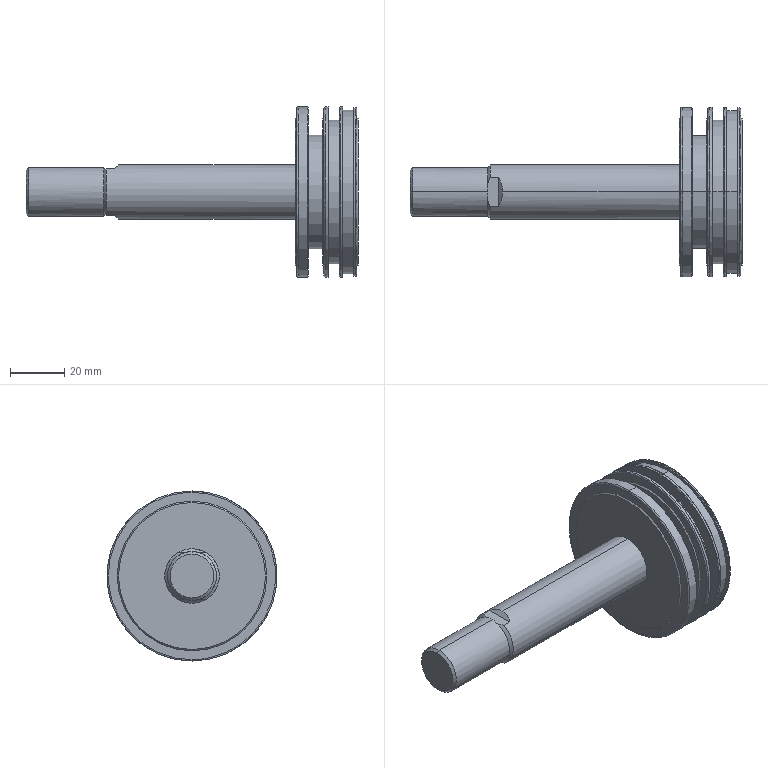Part | STEP file | ACQS_63x50-2 | 1 solid | 62 faces | box 122 x 62.5 x 62.5 mm | volume 85364 mm3 | cone 20 | cylinder 18 | plane 18 | spline 6 | commonest cylinder face diameters 62.5 x6 18 x2 20 x2 41.8 x2 52.9 x2 60 x2